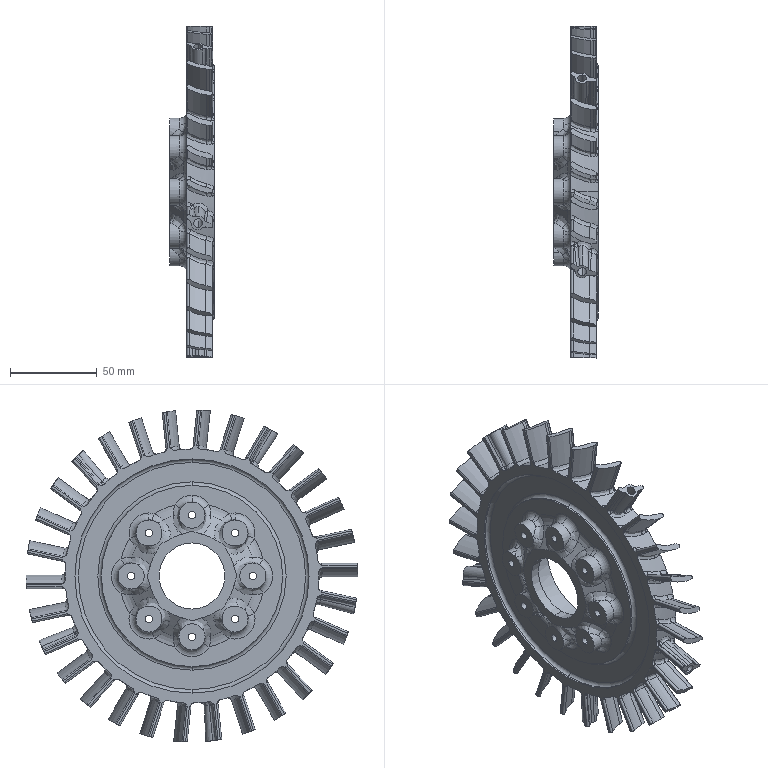Part | STEP file | 003.sldasm-Part-1_Valor predeterminado | 1 solid | 808 faces | box 26.301 x 191 x 190.919 mm | volume 221330 mm3 | cylinder 381 | spline 346 | sphere 30 | torus 27 | plane 16 | cone 8 | commonest cylinder face diameters 1.8 x90 17.78 x90 145.954 x36 52.324 x35 49.276 x30 191 x30